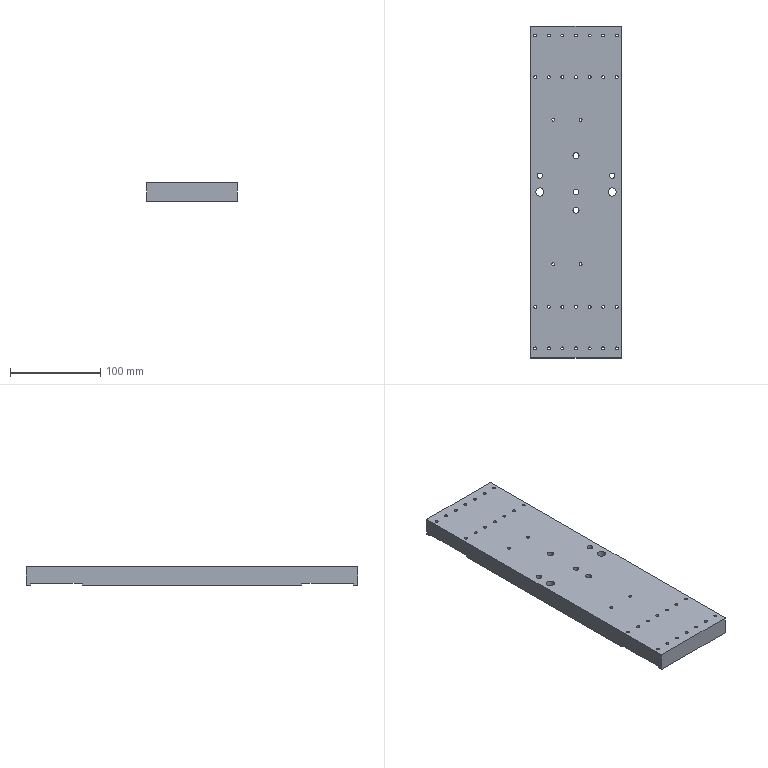CAM job | NX | 3-axis milling, drilling | part box 100 x 367 x 20 mm | stock box 100 x 372 x 25 mm
Tools:
number,name,description,diameter,corner_radius,flute_length,length,flutes
9,D10,平底铣刀-粗,10.0,0.0,35.0,75.0,2
10,D10-J,平底铣刀-精,10.0,0.0,35.0,75.0,2
1,D80R0.8_FACEMILL,圆鼻刀-粗,80.0,0.8,50.0,75.0,2
1,D80R0.8_FACEMILL-J,圆鼻刀-精,80.0,0.8,50.0,75.0,2
2,D6_CHAMFERMILL,倒角刀,6.0,0.0,3.0,25.0,2
21,M4X0.7,丝锥,3.3,0.0,35.0,50.0,2
22,M8X1.25,丝锥,6.8,0.0,35.0,50.0,2
23,D6_REAMER,Drilling Tool,6.0,0.0,75.0,100.0,6
13,ZT3.4,钻头,3.4,0.0,35.0,50.0,2
19,ZT9,钻头,9.0,0.0,35.0,50.0,2
17,ZT5.9,Drilling Tool,5.9,0.0,35.0,50.0,2
18,ZT6.9,Drilling Tool,6.9,0.0,35.0,50.0,2
Operations:
program,operation,operation_type,tool,method,geometry_group,spindle_rpm,surface_speed,feed_per_tooth,feed_cut,feed_plunge,cut_length_mm,path_length_mm,cut_time_min,machine_time_min
B,FLOORWALL_FACEROUGH_COPY,VolumeBased25DMillingOperation,D80R0.8_FACEMILL,LAYEREDROUGH-DEPTHK-STEPG,W-B,2800.0,703.696,0.5357,3000.0,100.0,8646.277,9096.854,2.882,2.927
B,FLOORWALL_FACEFINISH_COPY,VolumeBased25DMillingOperation,D80R0.8_FACEMILL-J,SIDEFINISH-DEPTHK-STEPG,W-B,4000.0,1005.28,0.125,1000.0,100.0,960.11,1056.11,0.9601,0.9697
B,NG_DRILLCHAMFER_2,Operation,D6_CHAMFERMILL,METHOD,W-B,8000.0,150.796,0.0625,1000.0,0.0,166.4,1321.196,0.1664,0.2819
B,MILLCHAMFER_4,PlanarMilling,D6_CHAMFERMILL,METHOD,W-B,8000.0,150.796,0.0375,600.0,100.0,56.866,450.05,0.0948,0.1341
B,MILLCHAMFER_5,PlanarMilling,D6_CHAMFERMILL,METHOD,W-B,8000.0,150.796,0.0375,600.0,100.0,62.549,322.149,0.1042,0.1302
B,MILLCHAMFER_6,PlanarMilling,D6_CHAMFERMILL,METHOD,W-B,8000.0,150.796,0.075,1200.0,100.0,46.839,334.096,0.039,0.0678
B,C0.3_CLOSEDCHAMFER6X45L_COPY,PlanarMilling,D6_CHAMFERMILL,SCALLOP_CHAMFER-DEPTH0-STEPG,W-B,7000.0,131.0,0.1071,1500.0,100.0,951.116,1047.117,0.6341,0.6437
A,TOPFACE,FaceMilling,D80R0.8_FACEMILL,SIDEFINISH-DEPTHK-STEPG,W-A,4500.0,1385.0,0.1667,1500.0,100.0,1445.0,1541.0,0.9633,0.9729
A,PROFILEROUGH_2,VolumeBased25DMillingOperation,D10,METHOD,W-A,8000.0,251.327,0.375,6000.0,80.0,26084.703,26203.203,4.348,4.359
A,FLOORWALLROUGH_1,VolumeBased25DMillingOperation,D10,METHOD,W-A,9000.0,282.743,0.3333,6000.0,100.0,7071.2,7751.333,1.179,1.246
A,SPOTDRILL-DEPTH0.8,Operation,D6_CHAMFERMILL,NONE,W-A,8000.0,150.796,0.0312,500.0,90.0,70.2,1223.801,0.1404,0.2558
A,THRUHOLE-M4TAPDRILL,Operation,ZT3.4,NONE,W-A,3000.0,31.102,0.05,300.0,90.0,864.0,2638.112,2.88,3.057
A,THRUHOLE-6.0PREDRILL,Operation,ZT5.9,NONE,W-A,2500.0,46.339,0.05,250.0,90.0,77.109,343.969,0.3084,0.3351
A,THRUHOLE-M8TAPDRILL,Operation,ZT6.9,NONE,W-A,1800.0,38.453,0.0972,350.0,90.0,60.0,281.008,0.1714,0.1935
A,THRUHOLE-8-10,Operation,ZT9,NONE,W-A,1800.0,50.894,0.0417,150.0,90.0,51.408,283.822,0.3427,0.366
A,FLOORFINISH_1,VolumeBased25DMillingOperation,D10-J,METHOD,W-A,9000.0,169.646,0.0833,1500.0,100.0,1773.4,2279.707,1.182,1.233
A,SOLIDONLY,SurfaceContour,D6_CHAMFERMILL,METHOD,W-A,8000.0,150.796,0.1875,3000.0,100.0,1409.494,3062.176,0.4698,0.6351
A,NG_DRILLCHAMFER_1,Operation,D6_CHAMFERMILL,METHOD,W-A,8000.0,150.796,0.0312,500.0,0.0,166.4,1311.863,0.3328,0.4473
A,MILLCHAMFER_1,PlanarMilling,D6_CHAMFERMILL,METHOD,W-A,8000.0,150.796,0.0312,500.0,100.0,62.891,453.718,0.1258,0.1649
A,MILLCHAMFER_2,PlanarMilling,D6_CHAMFERMILL,METHOD,W-A,8000.0,150.796,0.0375,600.0,100.0,48.803,315.002,0.0813,0.108
A,MILLCHAMFER_3,PlanarMilling,D6_CHAMFERMILL,METHOD,W-A,8000.0,150.796,0.05,800.0,100.0,69.821,352.004,0.0873,0.1155
A,FLOORSIDEFINISH_3,VolumeBased25DMillingOperation,D10-J,METHOD,W-A,9000.0,282.743,0.0556,1000.0,100.0,453.366,1274.843,0.4534,0.5355
A,REAM,Operation,D6_REAMER,METHOD,W-A,500.0,9.425,0.0167,50.0,0.0,66.0,321.75,1.32,1.346
A,THRUHOLE-TAPM4,Operation,M4X0.7,METHOD,W-A,600.0,6.22,0.0006,0.7,90.0,768.0,2442.034,1097.143,1097.31
A,THRUHOLE-TAPM8,Operation,M8X1.25,METHOD,W-A,500.0,10.681,0.0013,1.25,90.0,50.0,261.008,40.0,40.021
A,PROFILESEMIFINISH_2,VolumeBased25DMillingOperation,D10-J,METHOD,W-A,9000.0,169.646,0.0667,1200.0,100.0,1940.748,2201.263,1.617,1.643
A,FLOORWALLSIDEFINISH-MID_COPY,VolumeBased25DMillingOperation,D10-J,SIDEFINISH-DEPTHK-STEPG,W-A,8000.0,251.32,0.0625,1000.0,100.0,1538.256,2573.099,1.538,1.642